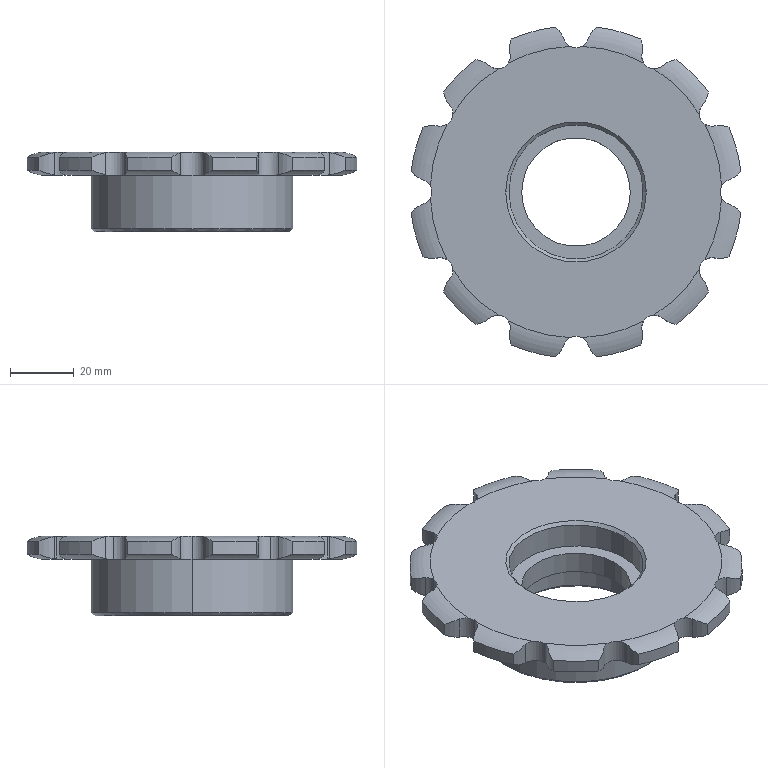Part | STEP file | 0228_105_Sprocket_RF2040S1200 | 1 solid | 98 faces | box 103.209 x 103.209 x 25 mm | volume 79551 mm3 | cylinder 63 | torus 24 | cone 6 | plane 5 | commonest cylinder face diameters 19.6 x26 7.92 x17 104 x12 42 x4 34 x2 63 x2